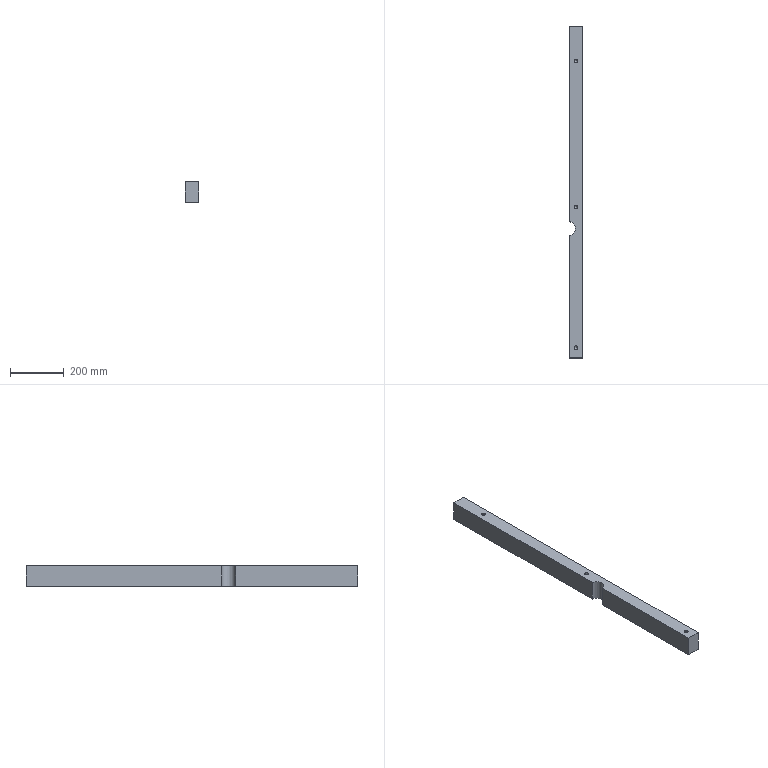Part | NX | features 3 2 | 1 solid | 20 faces | box 50 x 1233 x 75.5 mm | volume 4577587 mm3 | plane 7 | cylinder 7 | cone 6 | commonest cylinder face diameters 14.1 x6 53 x1
STEP:
#1=CARTESIAN_POINT('',(2567.05,542.5,256.5));
#2=VERTEX_POINT('',#1);
#3=CARTESIAN_POINT('',(2560.,542.5,256.5));
#4=DIRECTION('',(0.,0.,-1.));
#5=DIRECTION('',(1.,0.,0.));
#6=AXIS2_PLACEMENT_3D('',#3,#4,#5);
#7=CIRCLE('',#6,7.05);
#8=EDGE_CURVE('',#2,#2,#7,.T.);
#9=ORIENTED_EDGE('',*,*,#8,.T.);
#10=EDGE_LOOP('',(#9));
#11=FACE_BOUND('',#10,.T.);
#12=CARTESIAN_POINT('',(2535.,-53.804,256.5));
#13=VERTEX_POINT('',#12);
#14=CARTESIAN_POINT('',(2535.,-106.196,256.5));
#15=VERTEX_POINT('',#14);
#16=CARTESIAN_POINT('',(2531.,-80.,256.5));
#17=DIRECTION('',(0.,0.,-1.));
#18=DIRECTION('',(1.,0.,0.));
#19=AXIS2_PLACEMENT_3D('',#16,#17,#18);
#20=CIRCLE('',#19,26.5);
#21=EDGE_CURVE('',#13,#15,#20,.T.);
#22=ORIENTED_EDGE('',*,*,#21,.T.);
#23=CARTESIAN_POINT('',(2535.,-560.5,256.5));
#24=VERTEX_POINT('',#23);
#25=CARTESIAN_POINT('',(2535.,193.,256.5));
#26=DIRECTION('',(0.,-1.,0.));
#27=VECTOR('',#26,1000.);
#28=LINE('',#25,#27);
#29=EDGE_CURVE('',#15,#24,#28,.T.);
#30=ORIENTED_EDGE('',*,*,#29,.T.);
#31=CARTESIAN_POINT('',(2585.,-560.5,256.5));
#32=VERTEX_POINT('',#31);
#33=CARTESIAN_POINT('',(545.,-560.5,256.5));
#34=DIRECTION('',(1.,0.,0.));
#35=VECTOR('',#34,1000.);
#36=LINE('',#33,#35);
#37=EDGE_CURVE('',#24,#32,#36,.T.);
#38=ORIENTED_EDGE('',*,*,#37,.T.);
#39=CARTESIAN_POINT('',(2585.,672.5,256.5));
#40=VERTEX_POINT('',#39);
#41=CARTESIAN_POINT('',(2585.,193.,256.5));
#42=DIRECTION('',(0.,1.,0.));
#43=VECTOR('',#42,1000.);
#44=LINE('',#41,#43);
#45=EDGE_CURVE('',#32,#40,#44,.T.);
#46=ORIENTED_EDGE('',*,*,#45,.T.);
#47=CARTESIAN_POINT('',(2535.,672.5,256.5));
#48=VERTEX_POINT('',#47);
#49=CARTESIAN_POINT('',(545.,672.5,256.5));
#50=DIRECTION('',(-1.,0.,0.));
#51=VECTOR('',#50,1000.);
#52=LINE('',#49,#51);
#53=EDGE_CURVE('',#40,#48,#52,.T.);
#54=ORIENTED_EDGE('',*,*,#53,.T.);
#55=CARTESIAN_POINT('',(2535.,193.,256.5));
#56=DIRECTION('',(0.,-1.,0.));
#57=VECTOR('',#56,1000.);
#58=LINE('',#55,#57);
#59=EDGE_CURVE('',#48,#13,#58,.T.);
#60=ORIENTED_EDGE('',*,*,#59,.T.);
#61=EDGE_LOOP('',(#22,#30,#38,#46,#54,#60));
#62=FACE_BOUND('',#61,.T.);
#63=CARTESIAN_POINT('',(2567.05,0.,256.5));
#64=VERTEX_POINT('',#63);
#65=CARTESIAN_POINT('',(2560.,0.,256.5));
#66=DIRECTION('',(0.,0.,-1.));
#67=DIRECTION('',(1.,0.,0.));
#68=AXIS2_PLACEMENT_3D('',#65,#66,#67);
#69=CIRCLE('',#68,7.05);
#70=EDGE_CURVE('',#64,#64,#69,.T.);
#71=ORIENTED_EDGE('',*,*,#70,.T.);
#72=EDGE_LOOP('',(#71));
#73=FACE_BOUND('',#72,.T.);
#74=CARTESIAN_POINT('',(2567.05,-522.5,256.5));
#75=VERTEX_POINT('',#74);
#76=CARTESIAN_POINT('',(2560.,-522.5,256.5));
#77=DIRECTION('',(0.,0.,-1.));
#78=DIRECTION('',(1.,0.,0.));
#79=AXIS2_PLACEMENT_3D('',#76,#77,#78);
#80=CIRCLE('',#79,7.05);
#81=EDGE_CURVE('',#75,#75,#80,.T.);
#82=ORIENTED_EDGE('',*,*,#81,.T.);
#83=EDGE_LOOP('',(#82));
#84=FACE_BOUND('',#83,.T.);
#85=CARTESIAN_POINT('',(545.,0.,256.5));
#86=DIRECTION('',(0.,0.,1.));
#87=DIRECTION('',(1.,0.,0.));
#88=AXIS2_PLACEMENT_3D('',#85,#86,#87);
#89=PLANE('',#88);
#90=ADVANCED_FACE('',(#11,#62,#73,#84),#89,.T.);
#91=CARTESIAN_POINT('',(2567.05,-522.5,181.));
#92=VERTEX_POINT('',#91);
#93=CARTESIAN_POINT('',(2560.,-522.5,181.));
#94=DIRECTION('',(0.,0.,1.));
#95=DIRECTION('',(1.,0.,0.));
#96=AXIS2_PLACEMENT_3D('',#93,#94,#95);
#97=CIRCLE('',#96,7.05);
#98=EDGE_CURVE('',#92,#92,#97,.T.);
#99=ORIENTED_EDGE('',*,*,#98,.T.);
#100=EDGE_LOOP('',(#99));
#101=FACE_BOUND('',#100,.T.);
#102=CARTESIAN_POINT('',(2535.,-106.196,181.));
#103=VERTEX_POINT('',#102);
#104=CARTESIAN_POINT('',(2535.,-53.804,181.));
#105=VERTEX_POINT('',#104);
#106=CARTESIAN_POINT('',(2531.,-80.,181.));
#107=DIRECTION('',(0.,0.,1.));
#108=DIRECTION('',(-1.,0.,0.));
#109=AXIS2_PLACEMENT_3D('',#106,#107,#108);
#110=CIRCLE('',#109,26.5);
#111=EDGE_CURVE('',#103,#105,#110,.T.);
#112=ORIENTED_EDGE('',*,*,#111,.T.);
#113=CARTESIAN_POINT('',(2535.,672.5,181.));
#114=VERTEX_POINT('',#113);
#115=CARTESIAN_POINT('',(2535.,193.,181.));
#116=DIRECTION('',(0.,1.,0.));
#117=VECTOR('',#116,1000.);
#118=LINE('',#115,#117);
#119=EDGE_CURVE('',#105,#114,#118,.T.);
#120=ORIENTED_EDGE('',*,*,#119,.T.);
#121=CARTESIAN_POINT('',(2585.,672.5,181.));
#122=VERTEX_POINT('',#121);
#123=CARTESIAN_POINT('',(2585.,672.5,181.));
#124=DIRECTION('',(-1.,0.,0.));
#125=VECTOR('',#124,1000.);
#126=LINE('',#123,#125);
#127=EDGE_CURVE('',#122,#114,#126,.T.);
#128=ORIENTED_EDGE('',*,*,#127,.F.);
#129=CARTESIAN_POINT('',(2585.,-560.5,181.));
#130=VERTEX_POINT('',#129);
#131=CARTESIAN_POINT('',(2585.,193.,181.));
#132=DIRECTION('',(0.,-1.,0.));
#133=VECTOR('',#132,1000.);
#134=LINE('',#131,#133);
#135=EDGE_CURVE('',#122,#130,#134,.T.);
#136=ORIENTED_EDGE('',*,*,#135,.T.);
#137=CARTESIAN_POINT('',(2535.,-560.5,181.));
#138=VERTEX_POINT('',#137);
#139=CARTESIAN_POINT('',(1315.,-560.5,181.));
#140=DIRECTION('',(-1.,0.,0.));
#141=VECTOR('',#140,1000.);
#142=LINE('',#139,#141);
#143=EDGE_CURVE('',#130,#138,#142,.T.);
#144=ORIENTED_EDGE('',*,*,#143,.T.);
#145=CARTESIAN_POINT('',(2535.,193.,181.));
#146=DIRECTION('',(0.,1.,0.));
#147=VECTOR('',#146,1000.);
#148=LINE('',#145,#147);
#149=EDGE_CURVE('',#138,#103,#148,.T.);
#150=ORIENTED_EDGE('',*,*,#149,.T.);
#151=EDGE_LOOP('',(#112,#120,#128,#136,#144,#150));
#152=FACE_BOUND('',#151,.T.);
#153=CARTESIAN_POINT('',(2567.05,0.,181.));
#154=VERTEX_POINT('',#153);
#155=CARTESIAN_POINT('',(2560.,0.,181.));
#156=DIRECTION('',(0.,0.,1.));
#157=DIRECTION('',(1.,0.,0.));
#158=AXIS2_PLACEMENT_3D('',#155,#156,#157);
#159=CIRCLE('',#158,7.05);
#160=EDGE_CURVE('',#154,#154,#159,.T.);
#161=ORIENTED_EDGE('',*,*,#160,.T.);
#162=EDGE_LOOP('',(#161));
#163=FACE_BOUND('',#162,.T.);
#164=CARTESIAN_POINT('',(2567.05,542.5,181.));
#165=VERTEX_POINT('',#164);
#166=CARTESIAN_POINT('',(2560.,542.5,181.));
#167=DIRECTION('',(0.,0.,1.));
#168=DIRECTION('',(1.,0.,0.));
#169=AXIS2_PLACEMENT_3D('',#166,#167,#168);
#170=CIRCLE('',#169,7.05);
#171=EDGE_CURVE('',#165,#165,#170,.T.);
#172=ORIENTED_EDGE('',*,*,#171,.T.);
#173=EDGE_LOOP('',(#172));
#174=FACE_BOUND('',#173,.T.);
#175=CARTESIAN_POINT('',(1315.,193.,181.));
#176=DIRECTION('',(0.,0.,-1.));
#177=DIRECTION('',(1.,0.,0.));
#178=AXIS2_PLACEMENT_3D('',#175,#176,#177);
#179=PLANE('',#178);
#180=ADVANCED_FACE('',(#101,#152,#163,#174),#179,.T.);
#181=CARTESIAN_POINT('',(2535.,-106.196,-181.));
#182=DIRECTION('',(0.,0.,1.));
#183=VECTOR('',#182,1000.);
#184=LINE('',#181,#183);
#185=EDGE_CURVE('',#103,#15,#184,.T.);
#186=ORIENTED_EDGE('',*,*,#185,.F.);
#187=ORIENTED_EDGE('',*,*,#149,.F.);
#188=CARTESIAN_POINT('',(2535.,-560.5,-1.5));
#189=DIRECTION('',(0.,0.,1.));
#190=VECTOR('',#189,1000.);
#191=LINE('',#188,#190);
#192=EDGE_CURVE('',#138,#24,#191,.T.);
#193=ORIENTED_EDGE('',*,*,#192,.T.);
#194=ORIENTED_EDGE('',*,*,#29,.F.);
#195=EDGE_LOOP('',(#186,#187,#193,#194));
#196=FACE_BOUND('',#195,.T.);
#197=CARTESIAN_POINT('',(2535.,193.,-1.5));
#198=DIRECTION('',(-1.,0.,0.));
#199=DIRECTION('',(0.,0.,1.));
#200=AXIS2_PLACEMENT_3D('',#197,#198,#199);
#201=PLANE('',#200);
#202=ADVANCED_FACE('',(#196),#201,.T.);
#203=ORIENTED_EDGE('',*,*,#37,.F.);
#204=ORIENTED_EDGE('',*,*,#192,.F.);
#205=ORIENTED_EDGE('',*,*,#143,.F.);
#206=CARTESIAN_POINT('',(2585.,-560.5,-1.5));
#207=DIRECTION('',(0.,0.,-1.));
#208=VECTOR('',#207,1000.);
#209=LINE('',#206,#208);
#210=EDGE_CURVE('',#32,#130,#209,.T.);
#211=ORIENTED_EDGE('',*,*,#210,.F.);
#212=EDGE_LOOP('',(#203,#204,#205,#211));
#213=FACE_BOUND('',#212,.T.);
#214=CARTESIAN_POINT('',(2415.,-560.5,179.));
#215=DIRECTION('',(0.,-1.,0.));
#216=DIRECTION('',(-1.,0.,0.));
#217=AXIS2_PLACEMENT_3D('',#214,#215,#216);
#218=PLANE('',#217);
#219=ADVANCED_FACE('',(#213),#218,.T.);
#220=ORIENTED_EDGE('',*,*,#45,.F.);
#221=ORIENTED_EDGE('',*,*,#210,.T.);
#222=ORIENTED_EDGE('',*,*,#135,.F.);
#223=CARTESIAN_POINT('',(2585.,672.5,231.5));
#224=DIRECTION('',(0.,0.,-1.));
#225=VECTOR('',#224,1000.);
#226=LINE('',#223,#225);
#227=EDGE_CURVE('',#40,#122,#226,.T.);
#228=ORIENTED_EDGE('',*,*,#227,.F.);
#229=EDGE_LOOP('',(#220,#221,#222,#228));
#230=FACE_BOUND('',#229,.T.);
#231=CARTESIAN_POINT('',(2585.,193.,-1.5));
#232=DIRECTION('',(1.,0.,0.));
#233=DIRECTION('',(0.,0.,-1.));
#234=AXIS2_PLACEMENT_3D('',#231,#232,#233);
#235=PLANE('',#234);
#236=ADVANCED_FACE('',(#230),#235,.T.);
#237=CARTESIAN_POINT('',(2535.,-53.804,256.5));
#238=DIRECTION('',(0.,0.,-1.));
#239=VECTOR('',#238,1000.);
#240=LINE('',#237,#239);
#241=EDGE_CURVE('',#13,#105,#240,.T.);
#242=ORIENTED_EDGE('',*,*,#241,.F.);
#243=ORIENTED_EDGE('',*,*,#59,.F.);
#244=CARTESIAN_POINT('',(2535.,672.5,231.5));
#245=DIRECTION('',(0.,0.,1.));
#246=VECTOR('',#245,1000.);
#247=LINE('',#244,#246);
#248=EDGE_CURVE('',#114,#48,#247,.T.);
#249=ORIENTED_EDGE('',*,*,#248,.F.);
#250=ORIENTED_EDGE('',*,*,#119,.F.);
#251=EDGE_LOOP('',(#242,#243,#249,#250));
#252=FACE_BOUND('',#251,.T.);
#253=CARTESIAN_POINT('',(2535.,193.,-1.5));
#254=DIRECTION('',(-1.,0.,0.));
#255=DIRECTION('',(0.,0.,1.));
#256=AXIS2_PLACEMENT_3D('',#253,#254,#255);
#257=PLANE('',#256);
#258=ADVANCED_FACE('',(#252),#257,.T.);
#259=ORIENTED_EDGE('',*,*,#227,.T.);
#260=ORIENTED_EDGE('',*,*,#127,.T.);
#261=ORIENTED_EDGE('',*,*,#248,.T.);
#262=ORIENTED_EDGE('',*,*,#53,.F.);
#263=EDGE_LOOP('',(#259,#260,#261,#262));
#264=FACE_BOUND('',#263,.T.);
#265=CARTESIAN_POINT('',(2585.,672.5,231.5));
#266=DIRECTION('',(0.,1.,0.));
#267=DIRECTION('',(0.,0.,-1.));
#268=AXIS2_PLACEMENT_3D('',#265,#266,#267);
#269=PLANE('',#268);
#270=ADVANCED_FACE('',(#264),#269,.T.);
#271=ORIENTED_EDGE('',*,*,#21,.F.);
#272=ORIENTED_EDGE('',*,*,#241,.T.);
#273=ORIENTED_EDGE('',*,*,#111,.F.);
#274=ORIENTED_EDGE('',*,*,#185,.T.);
#275=EDGE_LOOP('',(#271,#272,#273,#274));
#276=FACE_BOUND('',#275,.T.);
#277=CARTESIAN_POINT('',(2531.,-80.,-181.));
#278=DIRECTION('',(0.,0.,1.));
#279=DIRECTION('',(-1.,0.,0.));
#280=AXIS2_PLACEMENT_3D('',#277,#278,#279);
#281=CYLINDRICAL_SURFACE('',#280,26.5);
#282=ADVANCED_FACE('',(#276),#281,.F.);
#283=CARTESIAN_POINT('',(2567.05,0.,188.95));
#284=VERTEX_POINT('',#283);
#285=CARTESIAN_POINT('',(2560.,0.,188.95));
#286=DIRECTION('',(0.,0.,1.));
#287=DIRECTION('',(1.,0.,0.));
#288=AXIS2_PLACEMENT_3D('',#285,#286,#287);
#289=CIRCLE('',#288,7.05);
#290=EDGE_CURVE('',#284,#284,#289,.T.);
#291=ORIENTED_EDGE('',*,*,#290,.T.);
#292=EDGE_LOOP('',(#291));
#293=FACE_BOUND('',#292,.T.);
#294=ORIENTED_EDGE('',*,*,#160,.F.);
#295=EDGE_LOOP('',(#294));
#296=FACE_BOUND('',#295,.T.);
#297=CARTESIAN_POINT('',(2560.,0.,181.));
#298=DIRECTION('',(0.,0.,1.));
#299=DIRECTION('',(-1.,0.,0.));
#300=AXIS2_PLACEMENT_3D('',#297,#298,#299);
#301=CYLINDRICAL_SURFACE('',#300,7.05);
#302=ADVANCED_FACE('',(#293,#296),#301,.F.);
#303=CARTESIAN_POINT('',(2560.,0.,196.));
#304=VERTEX_POINT('',#303);
#305=VERTEX_LOOP('',#304);
#306=FACE_BOUND('',#305,.T.);
#307=ORIENTED_EDGE('',*,*,#290,.F.);
#308=EDGE_LOOP('',(#307));
#309=FACE_BOUND('',#308,.T.);
#310=CARTESIAN_POINT('',(2560.,0.,188.95));
#311=DIRECTION('',(0.,0.,-1.));
#312=DIRECTION('',(1.,0.,0.));
#313=AXIS2_PLACEMENT_3D('',#310,#311,#312);
#314=CONICAL_SURFACE('',#313,7.05,0.7854);
#315=ADVANCED_FACE('',(#306,#309),#314,.F.);
#316=CARTESIAN_POINT('',(2567.05,-522.5,188.95));
#317=VERTEX_POINT('',#316);
#318=CARTESIAN_POINT('',(2560.,-522.5,188.95));
#319=DIRECTION('',(0.,0.,1.));
#320=DIRECTION('',(1.,0.,0.));
#321=AXIS2_PLACEMENT_3D('',#318,#319,#320);
#322=CIRCLE('',#321,7.05);
#323=EDGE_CURVE('',#317,#317,#322,.T.);
#324=ORIENTED_EDGE('',*,*,#323,.T.);
#325=EDGE_LOOP('',(#324));
#326=FACE_BOUND('',#325,.T.);
#327=ORIENTED_EDGE('',*,*,#98,.F.);
#328=EDGE_LOOP('',(#327));
#329=FACE_BOUND('',#328,.T.);
#330=CARTESIAN_POINT('',(2560.,-522.5,181.));
#331=DIRECTION('',(0.,0.,1.));
#332=DIRECTION('',(-1.,0.,0.));
#333=AXIS2_PLACEMENT_3D('',#330,#331,#332);
#334=CYLINDRICAL_SURFACE('',#333,7.05);
#335=ADVANCED_FACE('',(#326,#329),#334,.F.);
#336=CARTESIAN_POINT('',(2560.,-522.5,196.));
#337=VERTEX_POINT('',#336);
#338=VERTEX_LOOP('',#337);
#339=FACE_BOUND('',#338,.T.);
#340=ORIENTED_EDGE('',*,*,#323,.F.);
#341=EDGE_LOOP('',(#340));
#342=FACE_BOUND('',#341,.T.);
#343=CARTESIAN_POINT('',(2560.,-522.5,188.95));
#344=DIRECTION('',(0.,0.,-1.));
#345=DIRECTION('',(1.,0.,0.));
#346=AXIS2_PLACEMENT_3D('',#343,#344,#345);
#347=CONICAL_SURFACE('',#346,7.05,0.7854);
#348=ADVANCED_FACE('',(#339,#342),#347,.F.);
#349=CARTESIAN_POINT('',(2567.05,542.5,188.95));
#350=VERTEX_POINT('',#349);
#351=CARTESIAN_POINT('',(2560.,542.5,188.95));
#352=DIRECTION('',(0.,0.,1.));
#353=DIRECTION('',(1.,0.,0.));
#354=AXIS2_PLACEMENT_3D('',#351,#352,#353);
#355=CIRCLE('',#354,7.05);
#356=EDGE_CURVE('',#350,#350,#355,.T.);
#357=ORIENTED_EDGE('',*,*,#356,.T.);
#358=EDGE_LOOP('',(#357));
#359=FACE_BOUND('',#358,.T.);
#360=ORIENTED_EDGE('',*,*,#171,.F.);
#361=EDGE_LOOP('',(#360));
#362=FACE_BOUND('',#361,.T.);
#363=CARTESIAN_POINT('',(2560.,542.5,181.));
#364=DIRECTION('',(0.,0.,1.));
#365=DIRECTION('',(-1.,0.,0.));
#366=AXIS2_PLACEMENT_3D('',#363,#364,#365);
#367=CYLINDRICAL_SURFACE('',#366,7.05);
#368=ADVANCED_FACE('',(#359,#362),#367,.F.);
#369=CARTESIAN_POINT('',(2560.,542.5,196.));
#370=VERTEX_POINT('',#369);
#371=VERTEX_LOOP('',#370);
#372=FACE_BOUND('',#371,.T.);
#373=ORIENTED_EDGE('',*,*,#356,.F.);
#374=EDGE_LOOP('',(#373));
#375=FACE_BOUND('',#374,.T.);
#376=CARTESIAN_POINT('',(2560.,542.5,188.95));
#377=DIRECTION('',(0.,0.,-1.));
#378=DIRECTION('',(1.,0.,0.));
#379=AXIS2_PLACEMENT_3D('',#376,#377,#378);
#380=CONICAL_SURFACE('',#379,7.05,0.7854);
#381=ADVANCED_FACE('',(#372,#375),#380,.F.);
#382=CARTESIAN_POINT('',(2552.95,0.,248.55));
#383=VERTEX_POINT('',#382);
#384=CARTESIAN_POINT('',(2560.,0.,248.55));
#385=DIRECTION('',(0.,0.,-1.));
#386=DIRECTION('',(-1.,0.,0.));
#387=AXIS2_PLACEMENT_3D('',#384,#385,#386);
#388=CIRCLE('',#387,7.05);
#389=EDGE_CURVE('',#383,#383,#388,.T.);
#390=ORIENTED_EDGE('',*,*,#389,.T.);
#391=EDGE_LOOP('',(#390));
#392=FACE_BOUND('',#391,.T.);
#393=ORIENTED_EDGE('',*,*,#70,.F.);
#394=EDGE_LOOP('',(#393));
#395=FACE_BOUND('',#394,.T.);
#396=CARTESIAN_POINT('',(2560.,0.,256.5));
#397=DIRECTION('',(0.,0.,-1.));
#398=DIRECTION('',(-1.,0.,0.));
#399=AXIS2_PLACEMENT_3D('',#396,#397,#398);
#400=CYLINDRICAL_SURFACE('',#399,7.05);
#401=ADVANCED_FACE('',(#392,#395),#400,.F.);
#402=CARTESIAN_POINT('',(2560.,0.,241.5));
#403=VERTEX_POINT('',#402);
#404=VERTEX_LOOP('',#403);
#405=FACE_BOUND('',#404,.T.);
#406=ORIENTED_EDGE('',*,*,#389,.F.);
#407=EDGE_LOOP('',(#406));
#408=FACE_BOUND('',#407,.T.);
#409=CARTESIAN_POINT('',(2560.,0.,248.55));
#410=DIRECTION('',(0.,0.,1.));
#411=DIRECTION('',(-1.,0.,0.));
#412=AXIS2_PLACEMENT_3D('',#409,#410,#411);
#413=CONICAL_SURFACE('',#412,7.05,0.7854);
#414=ADVANCED_FACE('',(#405,#408),#413,.F.);
#415=CARTESIAN_POINT('',(2552.95,542.5,248.55));
#416=VERTEX_POINT('',#415);
#417=CARTESIAN_POINT('',(2560.,542.5,248.55));
#418=DIRECTION('',(0.,0.,-1.));
#419=DIRECTION('',(-1.,0.,0.));
#420=AXIS2_PLACEMENT_3D('',#417,#418,#419);
#421=CIRCLE('',#420,7.05);
#422=EDGE_CURVE('',#416,#416,#421,.T.);
#423=ORIENTED_EDGE('',*,*,#422,.T.);
#424=EDGE_LOOP('',(#423));
#425=FACE_BOUND('',#424,.T.);
#426=ORIENTED_EDGE('',*,*,#8,.F.);
#427=EDGE_LOOP('',(#426));
#428=FACE_BOUND('',#427,.T.);
#429=CARTESIAN_POINT('',(2560.,542.5,256.5));
#430=DIRECTION('',(0.,0.,-1.));
#431=DIRECTION('',(-1.,0.,0.));
#432=AXIS2_PLACEMENT_3D('',#429,#430,#431);
#433=CYLINDRICAL_SURFACE('',#432,7.05);
#434=ADVANCED_FACE('',(#425,#428),#433,.F.);
#435=CARTESIAN_POINT('',(2560.,542.5,241.5));
#436=VERTEX_POINT('',#435);
#437=VERTEX_LOOP('',#436);
#438=FACE_BOUND('',#437,.T.);
#439=ORIENTED_EDGE('',*,*,#422,.F.);
#440=EDGE_LOOP('',(#439));
#441=FACE_BOUND('',#440,.T.);
#442=CARTESIAN_POINT('',(2560.,542.5,248.55));
#443=DIRECTION('',(0.,0.,1.));
#444=DIRECTION('',(-1.,0.,0.));
#445=AXIS2_PLACEMENT_3D('',#442,#443,#444);
#446=CONICAL_SURFACE('',#445,7.05,0.7854);
#447=ADVANCED_FACE('',(#438,#441),#446,.F.);
#448=CARTESIAN_POINT('',(2552.95,-522.5,248.55));
#449=VERTEX_POINT('',#448);
#450=CARTESIAN_POINT('',(2560.,-522.5,248.55));
#451=DIRECTION('',(0.,0.,-1.));
#452=DIRECTION('',(-1.,0.,0.));
#453=AXIS2_PLACEMENT_3D('',#450,#451,#452);
#454=CIRCLE('',#453,7.05);
#455=EDGE_CURVE('',#449,#449,#454,.T.);
#456=ORIENTED_EDGE('',*,*,#455,.T.);
#457=EDGE_LOOP('',(#456));
#458=FACE_BOUND('',#457,.T.);
#459=ORIENTED_EDGE('',*,*,#81,.F.);
#460=EDGE_LOOP('',(#459));
#461=FACE_BOUND('',#460,.T.);
#462=CARTESIAN_POINT('',(2560.,-522.5,256.5));
#463=DIRECTION('',(0.,0.,-1.));
#464=DIRECTION('',(-1.,0.,0.));
#465=AXIS2_PLACEMENT_3D('',#462,#463,#464);
#466=CYLINDRICAL_SURFACE('',#465,7.05);
#467=ADVANCED_FACE('',(#458,#461),#466,.F.);
#468=CARTESIAN_POINT('',(2560.,-522.5,241.5));
#469=VERTEX_POINT('',#468);
#470=VERTEX_LOOP('',#469);
#471=FACE_BOUND('',#470,.T.);
#472=ORIENTED_EDGE('',*,*,#455,.F.);
#473=EDGE_LOOP('',(#472));
#474=FACE_BOUND('',#473,.T.);
#475=CARTESIAN_POINT('',(2560.,-522.5,248.55));
#476=DIRECTION('',(0.,0.,1.));
#477=DIRECTION('',(-1.,0.,0.));
#478=AXIS2_PLACEMENT_3D('',#475,#476,#477);
#479=CONICAL_SURFACE('',#478,7.05,0.7854);
#480=ADVANCED_FACE('',(#471,#474),#479,.F.);
#481=CLOSED_SHELL('',(#90,#180,#202,#219,#236,#258,#270,#282,#302,#315,#335,#348,#368,#381,#401,#414,#434,#447,#467,#480));
#482=MANIFOLD_SOLID_BREP('',#481);
#483=(LENGTH_UNIT()NAMED_UNIT(*)SI_UNIT(.MILLI.,.METRE.));
#484=UNCERTAINTY_MEASURE_WITH_UNIT(LENGTH_MEASURE(0.00001),#483,'','');
#485=(NAMED_UNIT(*)PLANE_ANGLE_UNIT()SI_UNIT($,.RADIAN.));
#486=(NAMED_UNIT(*)SI_UNIT($,.STERADIAN.)SOLID_ANGLE_UNIT());
#487=(GEOMETRIC_REPRESENTATION_CONTEXT(3)GLOBAL_UNCERTAINTY_ASSIGNED_CONTEXT((#484))GLOBAL_UNIT_ASSIGNED_CONTEXT((#483,#485,#486))REPRESENTATION_CONTEXT('',''));
#488=ADVANCED_BREP_SHAPE_REPRESENTATION('',(#482),#487);